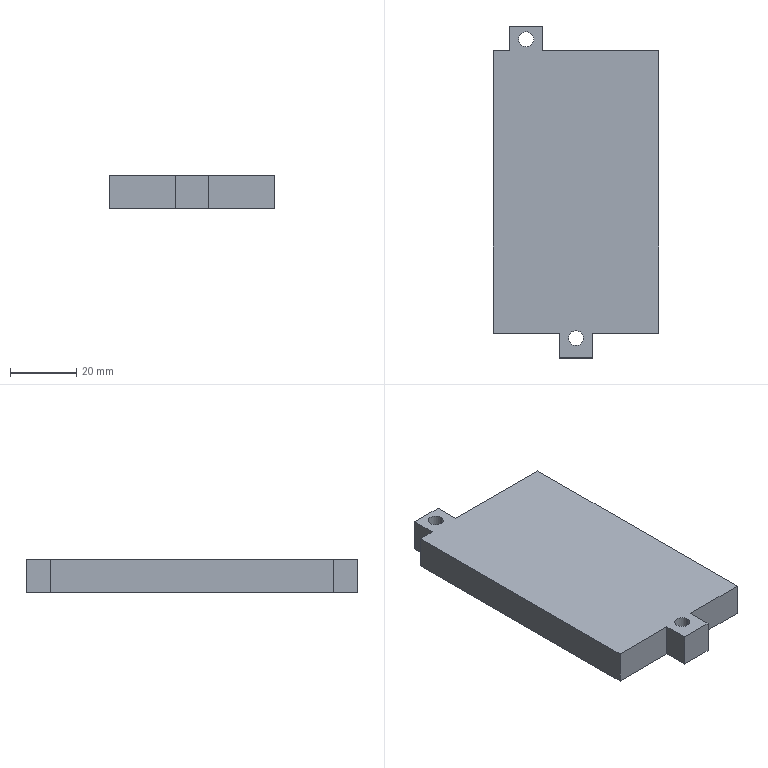Part | STEP file | Socket 1 | 1 solid | 18 faces | box 50 x 100 x 10 mm | volume 43682 mm3 | plane 14 | cylinder 4 | commonest cylinder face diameters 4.5 x4
STEP:
#1=CARTESIAN_POINT('',(0.,0.,0.));
#2=DIRECTION('',(0.,0.,1.));
#3=DIRECTION('',(1.,0.,0.));
#4=AXIS2_PLACEMENT_3D('',#1,#2,#3);
#5=CARTESIAN_POINT('',(-17.25,46.,10.));
#6=VERTEX_POINT('',#5);
#7=CARTESIAN_POINT('',(-17.25,46.,0.));
#8=VERTEX_POINT('',#7);
#9=CARTESIAN_POINT('',(-17.25,46.,10.));
#10=DIRECTION('',(0.,0.,-1.));
#11=VECTOR('',#10,1.);
#12=LINE('',#9,#11);
#13=CARTESIAN_POINT('',(-15.,46.,10.));
#14=DIRECTION('',(0.,0.,-1.));
#15=DIRECTION('',(-1.,0.,0.));
#16=AXIS2_PLACEMENT_3D('',#13,#14,#15);
#17=CYLINDRICAL_SURFACE('',#16,2.25);
#18=CARTESIAN_POINT('',(6.283,0.));
#19=DIRECTION('',(0.,1.));
#20=VECTOR('',#19,1.);
#21=LINE('',#18,#20);
#22=(GEOMETRIC_REPRESENTATION_CONTEXT(2)PARAMETRIC_REPRESENTATION_CONTEXT()REPRESENTATION_CONTEXT('',''));
#23=DEFINITIONAL_REPRESENTATION('',(#21),#22);
#24=PCURVE('',#17,#23);
#25=CARTESIAN_POINT('',(-15.,46.,10.));
#26=DIRECTION('',(0.,0.,-1.));
#27=DIRECTION('',(-1.,0.,0.));
#28=AXIS2_PLACEMENT_3D('',#25,#26,#27);
#29=CYLINDRICAL_SURFACE('',#28,2.25);
#30=CARTESIAN_POINT('',(0.,0.));
#31=DIRECTION('',(0.,1.));
#32=VECTOR('',#31,1.);
#33=LINE('',#30,#32);
#34=(GEOMETRIC_REPRESENTATION_CONTEXT(2)PARAMETRIC_REPRESENTATION_CONTEXT()REPRESENTATION_CONTEXT('',''));
#35=DEFINITIONAL_REPRESENTATION('',(#33),#34);
#36=PCURVE('',#29,#35);
#37=SURFACE_CURVE('',#12,(#24,#36),.PCURVE_S1.);
#38=EDGE_CURVE('',#6,#8,#37,.T.);
#39=ORIENTED_EDGE('',*,*,#38,.T.);
#40=CARTESIAN_POINT('',(-12.75,46.,0.));
#41=VERTEX_POINT('',#40);
#42=CARTESIAN_POINT('',(-15.,46.,0.));
#43=DIRECTION('',(0.,0.,1.));
#44=DIRECTION('',(-1.,0.,0.));
#45=AXIS2_PLACEMENT_3D('',#42,#43,#44);
#46=CIRCLE('',#45,2.25);
#47=CARTESIAN_POINT('',(6.283,10.));
#48=DIRECTION('',(-1.,0.));
#49=VECTOR('',#48,1.);
#50=LINE('',#47,#49);
#51=(GEOMETRIC_REPRESENTATION_CONTEXT(2)PARAMETRIC_REPRESENTATION_CONTEXT()REPRESENTATION_CONTEXT('',''));
#52=DEFINITIONAL_REPRESENTATION('',(#50),#51);
#53=PCURVE('',#17,#52);
#54=CARTESIAN_POINT('',(-1.349,-86.268,0.));
#55=DIRECTION('',(0.,0.,1.));
#56=DIRECTION('',(1.,0.,0.));
#57=AXIS2_PLACEMENT_3D('',#54,#55,#56);
#58=PLANE('',#57);
#59=CARTESIAN_POINT('',(-13.651,132.268));
#60=DIRECTION('',(-1.,0.));
#61=AXIS2_PLACEMENT_2D('',#59,#60);
#62=CIRCLE('',#61,2.25);
#63=(GEOMETRIC_REPRESENTATION_CONTEXT(2)PARAMETRIC_REPRESENTATION_CONTEXT()REPRESENTATION_CONTEXT('',''));
#64=DEFINITIONAL_REPRESENTATION('',(#62),#63);
#65=PCURVE('',#58,#64);
#66=SURFACE_CURVE('',#46,(#53,#65),.PCURVE_S1.);
#67=EDGE_CURVE('',#8,#41,#66,.T.);
#68=ORIENTED_EDGE('',*,*,#67,.T.);
#69=CARTESIAN_POINT('',(-12.75,46.,10.));
#70=VERTEX_POINT('',#69);
#71=CARTESIAN_POINT('',(-12.75,46.,10.));
#72=DIRECTION('',(0.,0.,-1.));
#73=VECTOR('',#72,1.);
#74=LINE('',#71,#73);
#75=CARTESIAN_POINT('',(3.142,0.));
#76=DIRECTION('',(0.,1.));
#77=VECTOR('',#76,1.);
#78=LINE('',#75,#77);
#79=(GEOMETRIC_REPRESENTATION_CONTEXT(2)PARAMETRIC_REPRESENTATION_CONTEXT()REPRESENTATION_CONTEXT('',''));
#80=DEFINITIONAL_REPRESENTATION('',(#78),#79);
#81=PCURVE('',#17,#80);
#82=CARTESIAN_POINT('',(3.142,0.));
#83=DIRECTION('',(0.,1.));
#84=VECTOR('',#83,1.);
#85=LINE('',#82,#84);
#86=(GEOMETRIC_REPRESENTATION_CONTEXT(2)PARAMETRIC_REPRESENTATION_CONTEXT()REPRESENTATION_CONTEXT('',''));
#87=DEFINITIONAL_REPRESENTATION('',(#85),#86);
#88=PCURVE('',#29,#87);
#89=SURFACE_CURVE('',#74,(#81,#88),.PCURVE_S1.);
#90=EDGE_CURVE('',#70,#41,#89,.T.);
#91=ORIENTED_EDGE('',*,*,#90,.F.);
#92=CARTESIAN_POINT('',(-15.,46.,10.));
#93=DIRECTION('',(0.,0.,-1.));
#94=DIRECTION('',(-1.,0.,0.));
#95=AXIS2_PLACEMENT_3D('',#92,#93,#94);
#96=CIRCLE('',#95,2.25);
#97=CARTESIAN_POINT('',(0.,0.));
#98=DIRECTION('',(1.,0.));
#99=VECTOR('',#98,1.);
#100=LINE('',#97,#99);
#101=(GEOMETRIC_REPRESENTATION_CONTEXT(2)PARAMETRIC_REPRESENTATION_CONTEXT()REPRESENTATION_CONTEXT('',''));
#102=DEFINITIONAL_REPRESENTATION('',(#100),#101);
#103=PCURVE('',#17,#102);
#104=CARTESIAN_POINT('',(-1.349,-86.268,10.));
#105=DIRECTION('',(0.,0.,1.));
#106=DIRECTION('',(1.,0.,0.));
#107=AXIS2_PLACEMENT_3D('',#104,#105,#106);
#108=PLANE('',#107);
#109=CARTESIAN_POINT('',(-15.901,132.268));
#110=CARTESIAN_POINT('',(-15.901,136.166));
#111=CARTESIAN_POINT('',(-12.526,134.217));
#112=CARTESIAN_POINT('',(-9.151,132.268));
#113=CARTESIAN_POINT('',(-12.526,130.32));
#114=CARTESIAN_POINT('',(-15.901,128.371));
#115=CARTESIAN_POINT('',(-15.901,132.268));
#116=(BOUNDED_CURVE()B_SPLINE_CURVE(2,(#109,#110,#111,#112,#113,#114,#115),.UNSPECIFIED.,.T.,.F.)B_SPLINE_CURVE_WITH_KNOTS((1,2,2,2,2,1),(-2.094,0.,2.094,4.189,6.283,8.378),.UNSPECIFIED.)CURVE()GEOMETRIC_REPRESENTATION_ITEM()RATIONAL_B_SPLINE_CURVE((1.,0.5,1.,0.5,1.,0.5,1.))REPRESENTATION_ITEM(''));
#117=(GEOMETRIC_REPRESENTATION_CONTEXT(2)PARAMETRIC_REPRESENTATION_CONTEXT()REPRESENTATION_CONTEXT('',''));
#118=DEFINITIONAL_REPRESENTATION('',(#116),#117);
#119=PCURVE('',#108,#118);
#120=SURFACE_CURVE('',#96,(#103,#119),.PCURVE_S1.);
#121=EDGE_CURVE('',#70,#6,#120,.T.);
#122=ORIENTED_EDGE('',*,*,#121,.T.);
#123=EDGE_LOOP('',(#39,#68,#91,#122));
#124=FACE_BOUND('',#123,.F.);
#125=ADVANCED_FACE('',(#124),#17,.F.);
#126=CARTESIAN_POINT('',(-2.25,-44.,10.));
#127=VERTEX_POINT('',#126);
#128=CARTESIAN_POINT('',(-2.25,-44.,0.));
#129=VERTEX_POINT('',#128);
#130=CARTESIAN_POINT('',(-2.25,-44.,10.));
#131=DIRECTION('',(0.,0.,-1.));
#132=VECTOR('',#131,1.);
#133=LINE('',#130,#132);
#134=CARTESIAN_POINT('',(0.,-44.,10.));
#135=DIRECTION('',(0.,0.,-1.));
#136=DIRECTION('',(-1.,0.,0.));
#137=AXIS2_PLACEMENT_3D('',#134,#135,#136);
#138=CYLINDRICAL_SURFACE('',#137,2.25);
#139=CARTESIAN_POINT('',(6.283,0.));
#140=DIRECTION('',(0.,1.));
#141=VECTOR('',#140,1.);
#142=LINE('',#139,#141);
#143=(GEOMETRIC_REPRESENTATION_CONTEXT(2)PARAMETRIC_REPRESENTATION_CONTEXT()REPRESENTATION_CONTEXT('',''));
#144=DEFINITIONAL_REPRESENTATION('',(#142),#143);
#145=PCURVE('',#138,#144);
#146=CARTESIAN_POINT('',(0.,-44.,10.));
#147=DIRECTION('',(0.,0.,-1.));
#148=DIRECTION('',(-1.,0.,0.));
#149=AXIS2_PLACEMENT_3D('',#146,#147,#148);
#150=CYLINDRICAL_SURFACE('',#149,2.25);
#151=CARTESIAN_POINT('',(0.,0.));
#152=DIRECTION('',(0.,1.));
#153=VECTOR('',#152,1.);
#154=LINE('',#151,#153);
#155=(GEOMETRIC_REPRESENTATION_CONTEXT(2)PARAMETRIC_REPRESENTATION_CONTEXT()REPRESENTATION_CONTEXT('',''));
#156=DEFINITIONAL_REPRESENTATION('',(#154),#155);
#157=PCURVE('',#150,#156);
#158=SURFACE_CURVE('',#133,(#145,#157),.PCURVE_S1.);
#159=EDGE_CURVE('',#127,#129,#158,.T.);
#160=ORIENTED_EDGE('',*,*,#159,.T.);
#161=CARTESIAN_POINT('',(2.25,-44.,0.));
#162=VERTEX_POINT('',#161);
#163=CARTESIAN_POINT('',(0.,-44.,0.));
#164=DIRECTION('',(0.,0.,1.));
#165=DIRECTION('',(-1.,0.,0.));
#166=AXIS2_PLACEMENT_3D('',#163,#164,#165);
#167=CIRCLE('',#166,2.25);
#168=CARTESIAN_POINT('',(6.283,10.));
#169=DIRECTION('',(-1.,0.));
#170=VECTOR('',#169,1.);
#171=LINE('',#168,#170);
#172=(GEOMETRIC_REPRESENTATION_CONTEXT(2)PARAMETRIC_REPRESENTATION_CONTEXT()REPRESENTATION_CONTEXT('',''));
#173=DEFINITIONAL_REPRESENTATION('',(#171),#172);
#174=PCURVE('',#138,#173);
#175=CARTESIAN_POINT('',(1.349,42.268));
#176=DIRECTION('',(-1.,0.));
#177=AXIS2_PLACEMENT_2D('',#175,#176);
#178=CIRCLE('',#177,2.25);
#179=(GEOMETRIC_REPRESENTATION_CONTEXT(2)PARAMETRIC_REPRESENTATION_CONTEXT()REPRESENTATION_CONTEXT('',''));
#180=DEFINITIONAL_REPRESENTATION('',(#178),#179);
#181=PCURVE('',#58,#180);
#182=SURFACE_CURVE('',#167,(#174,#181),.PCURVE_S1.);
#183=EDGE_CURVE('',#129,#162,#182,.T.);
#184=ORIENTED_EDGE('',*,*,#183,.T.);
#185=CARTESIAN_POINT('',(2.25,-44.,10.));
#186=VERTEX_POINT('',#185);
#187=CARTESIAN_POINT('',(2.25,-44.,10.));
#188=DIRECTION('',(0.,0.,-1.));
#189=VECTOR('',#188,1.);
#190=LINE('',#187,#189);
#191=CARTESIAN_POINT('',(3.142,0.));
#192=DIRECTION('',(0.,1.));
#193=VECTOR('',#192,1.);
#194=LINE('',#191,#193);
#195=(GEOMETRIC_REPRESENTATION_CONTEXT(2)PARAMETRIC_REPRESENTATION_CONTEXT()REPRESENTATION_CONTEXT('',''));
#196=DEFINITIONAL_REPRESENTATION('',(#194),#195);
#197=PCURVE('',#138,#196);
#198=CARTESIAN_POINT('',(3.142,0.));
#199=DIRECTION('',(0.,1.));
#200=VECTOR('',#199,1.);
#201=LINE('',#198,#200);
#202=(GEOMETRIC_REPRESENTATION_CONTEXT(2)PARAMETRIC_REPRESENTATION_CONTEXT()REPRESENTATION_CONTEXT('',''));
#203=DEFINITIONAL_REPRESENTATION('',(#201),#202);
#204=PCURVE('',#150,#203);
#205=SURFACE_CURVE('',#190,(#197,#204),.PCURVE_S1.);
#206=EDGE_CURVE('',#186,#162,#205,.T.);
#207=ORIENTED_EDGE('',*,*,#206,.F.);
#208=CARTESIAN_POINT('',(0.,-44.,10.));
#209=DIRECTION('',(0.,0.,-1.));
#210=DIRECTION('',(-1.,0.,0.));
#211=AXIS2_PLACEMENT_3D('',#208,#209,#210);
#212=CIRCLE('',#211,2.25);
#213=CARTESIAN_POINT('',(0.,0.));
#214=DIRECTION('',(1.,0.));
#215=VECTOR('',#214,1.);
#216=LINE('',#213,#215);
#217=(GEOMETRIC_REPRESENTATION_CONTEXT(2)PARAMETRIC_REPRESENTATION_CONTEXT()REPRESENTATION_CONTEXT('',''));
#218=DEFINITIONAL_REPRESENTATION('',(#216),#217);
#219=PCURVE('',#138,#218);
#220=CARTESIAN_POINT('',(-0.9015,42.268));
#221=CARTESIAN_POINT('',(-0.9015,46.166));
#222=CARTESIAN_POINT('',(2.474,44.217));
#223=CARTESIAN_POINT('',(5.849,42.268));
#224=CARTESIAN_POINT('',(2.474,40.32));
#225=CARTESIAN_POINT('',(-0.9015,38.371));
#226=CARTESIAN_POINT('',(-0.9015,42.268));
#227=(BOUNDED_CURVE()B_SPLINE_CURVE(2,(#220,#221,#222,#223,#224,#225,#226),.UNSPECIFIED.,.T.,.F.)B_SPLINE_CURVE_WITH_KNOTS((1,2,2,2,2,1),(-2.094,0.,2.094,4.189,6.283,8.378),.UNSPECIFIED.)CURVE()GEOMETRIC_REPRESENTATION_ITEM()RATIONAL_B_SPLINE_CURVE((1.,0.5,1.,0.5,1.,0.5,1.))REPRESENTATION_ITEM(''));
#228=(GEOMETRIC_REPRESENTATION_CONTEXT(2)PARAMETRIC_REPRESENTATION_CONTEXT()REPRESENTATION_CONTEXT('',''));
#229=DEFINITIONAL_REPRESENTATION('',(#227),#228);
#230=PCURVE('',#108,#229);
#231=SURFACE_CURVE('',#212,(#219,#230),.PCURVE_S1.);
#232=EDGE_CURVE('',#186,#127,#231,.T.);
#233=ORIENTED_EDGE('',*,*,#232,.T.);
#234=EDGE_LOOP('',(#160,#184,#207,#233));
#235=FACE_BOUND('',#234,.F.);
#236=ADVANCED_FACE('',(#235),#138,.F.);
#237=CARTESIAN_POINT('',(-15.,46.,10.));
#238=DIRECTION('',(0.,0.,-1.));
#239=DIRECTION('',(-1.,0.,0.));
#240=AXIS2_PLACEMENT_3D('',#237,#238,#239);
#241=CIRCLE('',#240,2.25);
#242=CARTESIAN_POINT('',(-15.901,132.268));
#243=CARTESIAN_POINT('',(-15.901,136.166));
#244=CARTESIAN_POINT('',(-12.526,134.217));
#245=CARTESIAN_POINT('',(-9.151,132.268));
#246=CARTESIAN_POINT('',(-12.526,130.32));
#247=CARTESIAN_POINT('',(-15.901,128.371));
#248=CARTESIAN_POINT('',(-15.901,132.268));
#249=(BOUNDED_CURVE()B_SPLINE_CURVE(2,(#242,#243,#244,#245,#246,#247,#248),.UNSPECIFIED.,.T.,.F.)B_SPLINE_CURVE_WITH_KNOTS((1,2,2,2,2,1),(-2.094,0.,2.094,4.189,6.283,8.378),.UNSPECIFIED.)CURVE()GEOMETRIC_REPRESENTATION_ITEM()RATIONAL_B_SPLINE_CURVE((1.,0.5,1.,0.5,1.,0.5,1.))REPRESENTATION_ITEM(''));
#250=(GEOMETRIC_REPRESENTATION_CONTEXT(2)PARAMETRIC_REPRESENTATION_CONTEXT()REPRESENTATION_CONTEXT('',''));
#251=DEFINITIONAL_REPRESENTATION('',(#249),#250);
#252=PCURVE('',#108,#251);
#253=CARTESIAN_POINT('',(0.,0.));
#254=DIRECTION('',(1.,0.));
#255=VECTOR('',#254,1.);
#256=LINE('',#253,#255);
#257=(GEOMETRIC_REPRESENTATION_CONTEXT(2)PARAMETRIC_REPRESENTATION_CONTEXT()REPRESENTATION_CONTEXT('',''));
#258=DEFINITIONAL_REPRESENTATION('',(#256),#257);
#259=PCURVE('',#29,#258);
#260=SURFACE_CURVE('',#241,(#252,#259),.PCURVE_S1.);
#261=EDGE_CURVE('',#6,#70,#260,.T.);
#262=ORIENTED_EDGE('',*,*,#261,.T.);
#263=ORIENTED_EDGE('',*,*,#121,.T.);
#264=EDGE_LOOP('',(#262,#263));
#265=FACE_BOUND('',#264,.T.);
#266=CARTESIAN_POINT('',(0.,-44.,10.));
#267=DIRECTION('',(0.,0.,-1.));
#268=DIRECTION('',(-1.,0.,0.));
#269=AXIS2_PLACEMENT_3D('',#266,#267,#268);
#270=CIRCLE('',#269,2.25);
#271=CARTESIAN_POINT('',(-0.9015,42.268));
#272=CARTESIAN_POINT('',(-0.9015,46.166));
#273=CARTESIAN_POINT('',(2.474,44.217));
#274=CARTESIAN_POINT('',(5.849,42.268));
#275=CARTESIAN_POINT('',(2.474,40.32));
#276=CARTESIAN_POINT('',(-0.9015,38.371));
#277=CARTESIAN_POINT('',(-0.9015,42.268));
#278=(BOUNDED_CURVE()B_SPLINE_CURVE(2,(#271,#272,#273,#274,#275,#276,#277),.UNSPECIFIED.,.T.,.F.)B_SPLINE_CURVE_WITH_KNOTS((1,2,2,2,2,1),(-2.094,0.,2.094,4.189,6.283,8.378),.UNSPECIFIED.)CURVE()GEOMETRIC_REPRESENTATION_ITEM()RATIONAL_B_SPLINE_CURVE((1.,0.5,1.,0.5,1.,0.5,1.))REPRESENTATION_ITEM(''));
#279=(GEOMETRIC_REPRESENTATION_CONTEXT(2)PARAMETRIC_REPRESENTATION_CONTEXT()REPRESENTATION_CONTEXT('',''));
#280=DEFINITIONAL_REPRESENTATION('',(#278),#279);
#281=PCURVE('',#108,#280);
#282=CARTESIAN_POINT('',(0.,0.));
#283=DIRECTION('',(1.,0.));
#284=VECTOR('',#283,1.);
#285=LINE('',#282,#284);
#286=(GEOMETRIC_REPRESENTATION_CONTEXT(2)PARAMETRIC_REPRESENTATION_CONTEXT()REPRESENTATION_CONTEXT('',''));
#287=DEFINITIONAL_REPRESENTATION('',(#285),#286);
#288=PCURVE('',#150,#287);
#289=SURFACE_CURVE('',#270,(#281,#288),.PCURVE_S1.);
#290=EDGE_CURVE('',#127,#186,#289,.T.);
#291=ORIENTED_EDGE('',*,*,#290,.T.);
#292=ORIENTED_EDGE('',*,*,#232,.T.);
#293=EDGE_LOOP('',(#291,#292));
#294=FACE_BOUND('',#293,.T.);
#295=CARTESIAN_POINT('',(-5.,-42.5,10.));
#296=VERTEX_POINT('',#295);
#297=CARTESIAN_POINT('',(-5.,-50.,10.));
#298=VERTEX_POINT('',#297);
#299=CARTESIAN_POINT('',(-5.,-86.268,10.));
#300=DIRECTION('',(0.,-1.,0.));
#301=VECTOR('',#300,1.);
#302=LINE('',#299,#301);
#303=CARTESIAN_POINT('',(-3.651,0.));
#304=DIRECTION('',(0.,-1.));
#305=VECTOR('',#304,1.);
#306=LINE('',#303,#305);
#307=(GEOMETRIC_REPRESENTATION_CONTEXT(2)PARAMETRIC_REPRESENTATION_CONTEXT()REPRESENTATION_CONTEXT('',''));
#308=DEFINITIONAL_REPRESENTATION('',(#306),#307);
#309=PCURVE('',#108,#308);
#310=CARTESIAN_POINT('',(-5.,-86.268,10.));
#311=DIRECTION('',(1.,0.,0.));
#312=DIRECTION('',(0.,1.,0.));
#313=AXIS2_PLACEMENT_3D('',#310,#311,#312);
#314=PLANE('',#313);
#315=CARTESIAN_POINT('',(0.,0.));
#316=DIRECTION('',(-1.,0.));
#317=VECTOR('',#316,1.);
#318=LINE('',#315,#317);
#319=(GEOMETRIC_REPRESENTATION_CONTEXT(2)PARAMETRIC_REPRESENTATION_CONTEXT()REPRESENTATION_CONTEXT('',''));
#320=DEFINITIONAL_REPRESENTATION('',(#318),#319);
#321=PCURVE('',#314,#320);
#322=SURFACE_CURVE('',#302,(#309,#321),.PCURVE_S1.);
#323=EDGE_CURVE('',#296,#298,#322,.T.);
#324=ORIENTED_EDGE('',*,*,#323,.T.);
#325=CARTESIAN_POINT('',(5.,-50.,10.));
#326=VERTEX_POINT('',#325);
#327=CARTESIAN_POINT('',(-1.349,-50.,10.));
#328=DIRECTION('',(1.,0.,0.));
#329=VECTOR('',#328,1.);
#330=LINE('',#327,#329);
#331=CARTESIAN_POINT('',(0.,36.268));
#332=DIRECTION('',(1.,0.));
#333=VECTOR('',#332,1.);
#334=LINE('',#331,#333);
#335=(GEOMETRIC_REPRESENTATION_CONTEXT(2)PARAMETRIC_REPRESENTATION_CONTEXT()REPRESENTATION_CONTEXT('',''));
#336=DEFINITIONAL_REPRESENTATION('',(#334),#335);
#337=PCURVE('',#108,#336);
#338=CARTESIAN_POINT('',(-1.349,-50.,10.));
#339=DIRECTION('',(0.,1.,0.));
#340=DIRECTION('',(0.,0.,1.));
#341=AXIS2_PLACEMENT_3D('',#338,#339,#340);
#342=PLANE('',#341);
#343=CARTESIAN_POINT('',(0.,0.));
#344=DIRECTION('',(0.,1.));
#345=VECTOR('',#344,1.);
#346=LINE('',#343,#345);
#347=(GEOMETRIC_REPRESENTATION_CONTEXT(2)PARAMETRIC_REPRESENTATION_CONTEXT()REPRESENTATION_CONTEXT('',''));
#348=DEFINITIONAL_REPRESENTATION('',(#346),#347);
#349=PCURVE('',#342,#348);
#350=SURFACE_CURVE('',#330,(#337,#349),.PCURVE_S1.);
#351=EDGE_CURVE('',#298,#326,#350,.T.);
#352=ORIENTED_EDGE('',*,*,#351,.T.);
#353=CARTESIAN_POINT('',(5.,-42.5,10.));
#354=VERTEX_POINT('',#353);
#355=CARTESIAN_POINT('',(5.,-86.268,10.));
#356=DIRECTION('',(0.,1.,0.));
#357=VECTOR('',#356,1.);
#358=LINE('',#355,#357);
#359=CARTESIAN_POINT('',(6.349,0.));
#360=DIRECTION('',(0.,1.));
#361=VECTOR('',#360,1.);
#362=LINE('',#359,#361);
#363=(GEOMETRIC_REPRESENTATION_CONTEXT(2)PARAMETRIC_REPRESENTATION_CONTEXT()REPRESENTATION_CONTEXT('',''));
#364=DEFINITIONAL_REPRESENTATION('',(#362),#363);
#365=PCURVE('',#108,#364);
#366=CARTESIAN_POINT('',(5.,-86.268,10.));
#367=DIRECTION('',(1.,0.,0.));
#368=DIRECTION('',(0.,1.,0.));
#369=AXIS2_PLACEMENT_3D('',#366,#367,#368);
#370=PLANE('',#369);
#371=CARTESIAN_POINT('',(0.,0.));
#372=DIRECTION('',(1.,0.));
#373=VECTOR('',#372,1.);
#374=LINE('',#371,#373);
#375=(GEOMETRIC_REPRESENTATION_CONTEXT(2)PARAMETRIC_REPRESENTATION_CONTEXT()REPRESENTATION_CONTEXT('',''));
#376=DEFINITIONAL_REPRESENTATION('',(#374),#375);
#377=PCURVE('',#370,#376);
#378=SURFACE_CURVE('',#358,(#365,#377),.PCURVE_S1.);
#379=EDGE_CURVE('',#326,#354,#378,.T.);
#380=ORIENTED_EDGE('',*,*,#379,.T.);
#381=CARTESIAN_POINT('',(25.,-42.5,10.));
#382=VERTEX_POINT('',#381);
#383=CARTESIAN_POINT('',(-1.349,-42.5,10.));
#384=DIRECTION('',(1.,0.,0.));
#385=VECTOR('',#384,1.);
#386=LINE('',#383,#385);
#387=CARTESIAN_POINT('',(0.,43.768));
#388=DIRECTION('',(1.,0.));
#389=VECTOR('',#388,1.);
#390=LINE('',#387,#389);
#391=(GEOMETRIC_REPRESENTATION_CONTEXT(2)PARAMETRIC_REPRESENTATION_CONTEXT()REPRESENTATION_CONTEXT('',''));
#392=DEFINITIONAL_REPRESENTATION('',(#390),#391);
#393=PCURVE('',#108,#392);
#394=CARTESIAN_POINT('',(-1.349,-42.5,10.));
#395=DIRECTION('',(0.,1.,0.));
#396=DIRECTION('',(0.,0.,1.));
#397=AXIS2_PLACEMENT_3D('',#394,#395,#396);
#398=PLANE('',#397);
#399=CARTESIAN_POINT('',(0.,0.));
#400=DIRECTION('',(0.,1.));
#401=VECTOR('',#400,1.);
#402=LINE('',#399,#401);
#403=(GEOMETRIC_REPRESENTATION_CONTEXT(2)PARAMETRIC_REPRESENTATION_CONTEXT()REPRESENTATION_CONTEXT('',''));
#404=DEFINITIONAL_REPRESENTATION('',(#402),#403);
#405=PCURVE('',#398,#404);
#406=SURFACE_CURVE('',#386,(#393,#405),.PCURVE_S1.);
#407=EDGE_CURVE('',#354,#382,#406,.T.);
#408=ORIENTED_EDGE('',*,*,#407,.T.);
#409=CARTESIAN_POINT('',(25.,42.5,10.));
#410=VERTEX_POINT('',#409);
#411=CARTESIAN_POINT('',(25.,-86.268,10.));
#412=DIRECTION('',(0.,1.,0.));
#413=VECTOR('',#412,1.);
#414=LINE('',#411,#413);
#415=CARTESIAN_POINT('',(26.349,0.));
#416=DIRECTION('',(0.,1.));
#417=VECTOR('',#416,1.);
#418=LINE('',#415,#417);
#419=(GEOMETRIC_REPRESENTATION_CONTEXT(2)PARAMETRIC_REPRESENTATION_CONTEXT()REPRESENTATION_CONTEXT('',''));
#420=DEFINITIONAL_REPRESENTATION('',(#418),#419);
#421=PCURVE('',#108,#420);
#422=CARTESIAN_POINT('',(25.,-86.268,10.));
#423=DIRECTION('',(1.,0.,0.));
#424=DIRECTION('',(0.,1.,0.));
#425=AXIS2_PLACEMENT_3D('',#422,#423,#424);
#426=PLANE('',#425);
#427=CARTESIAN_POINT('',(0.,0.));
#428=DIRECTION('',(1.,0.));
#429=VECTOR('',#428,1.);
#430=LINE('',#427,#429);
#431=(GEOMETRIC_REPRESENTATION_CONTEXT(2)PARAMETRIC_REPRESENTATION_CONTEXT()REPRESENTATION_CONTEXT('',''));
#432=DEFINITIONAL_REPRESENTATION('',(#430),#431);
#433=PCURVE('',#426,#432);
#434=SURFACE_CURVE('',#414,(#421,#433),.PCURVE_S1.);
#435=EDGE_CURVE('',#382,#410,#434,.T.);
#436=ORIENTED_EDGE('',*,*,#435,.T.);
#437=CARTESIAN_POINT('',(-10.,42.5,10.));
#438=VERTEX_POINT('',#437);
#439=CARTESIAN_POINT('',(-1.349,42.5,10.));
#440=DIRECTION('',(-1.,0.,0.));
#441=VECTOR('',#440,1.);
#442=LINE('',#439,#441);
#443=CARTESIAN_POINT('',(0.,128.768));
#444=DIRECTION('',(-1.,0.));
#445=VECTOR('',#444,1.);
#446=LINE('',#443,#445);
#447=(GEOMETRIC_REPRESENTATION_CONTEXT(2)PARAMETRIC_REPRESENTATION_CONTEXT()REPRESENTATION_CONTEXT('',''));
#448=DEFINITIONAL_REPRESENTATION('',(#446),#447);
#449=PCURVE('',#108,#448);
#450=CARTESIAN_POINT('',(-1.349,42.5,10.));
#451=DIRECTION('',(0.,1.,0.));
#452=DIRECTION('',(0.,0.,1.));
#453=AXIS2_PLACEMENT_3D('',#450,#451,#452);
#454=PLANE('',#453);
#455=CARTESIAN_POINT('',(0.,0.));
#456=DIRECTION('',(0.,-1.));
#457=VECTOR('',#456,1.);
#458=LINE('',#455,#457);
#459=(GEOMETRIC_REPRESENTATION_CONTEXT(2)PARAMETRIC_REPRESENTATION_CONTEXT()REPRESENTATION_CONTEXT('',''));
#460=DEFINITIONAL_REPRESENTATION('',(#458),#459);
#461=PCURVE('',#454,#460);
#462=SURFACE_CURVE('',#442,(#449,#461),.PCURVE_S1.);
#463=EDGE_CURVE('',#410,#438,#462,.T.);
#464=ORIENTED_EDGE('',*,*,#463,.T.);
#465=CARTESIAN_POINT('',(-10.,50.,10.));
#466=VERTEX_POINT('',#465);
#467=CARTESIAN_POINT('',(-10.,-86.268,10.));
#468=DIRECTION('',(0.,1.,0.));
#469=VECTOR('',#468,1.);
#470=LINE('',#467,#469);
#471=CARTESIAN_POINT('',(-8.651,0.));
#472=DIRECTION('',(0.,1.));
#473=VECTOR('',#472,1.);
#474=LINE('',#471,#473);
#475=(GEOMETRIC_REPRESENTATION_CONTEXT(2)PARAMETRIC_REPRESENTATION_CONTEXT()REPRESENTATION_CONTEXT('',''));
#476=DEFINITIONAL_REPRESENTATION('',(#474),#475);
#477=PCURVE('',#108,#476);
#478=CARTESIAN_POINT('',(-10.,-86.268,10.));
#479=DIRECTION('',(-1.,0.,0.));
#480=DIRECTION('',(0.,-1.,0.));
#481=AXIS2_PLACEMENT_3D('',#478,#479,#480);
#482=PLANE('',#481);
#483=CARTESIAN_POINT('',(0.,0.));
#484=DIRECTION('',(-1.,0.));
#485=VECTOR('',#484,1.);
#486=LINE('',#483,#485);
#487=(GEOMETRIC_REPRESENTATION_CONTEXT(2)PARAMETRIC_REPRESENTATION_CONTEXT()REPRESENTATION_CONTEXT('',''));
#488=DEFINITIONAL_REPRESENTATION('',(#486),#487);
#489=PCURVE('',#482,#488);
#490=SURFACE_CURVE('',#470,(#477,#489),.PCURVE_S1.);
#491=EDGE_CURVE('',#438,#466,#490,.T.);
#492=ORIENTED_EDGE('',*,*,#491,.T.);
#493=CARTESIAN_POINT('',(-20.,50.,10.));
#494=VERTEX_POINT('',#493);
#495=CARTESIAN_POINT('',(-1.349,50.,10.));
#496=DIRECTION('',(-1.,0.,0.));
#497=VECTOR('',#496,1.);
#498=LINE('',#495,#497);
#499=CARTESIAN_POINT('',(0.,136.268));
#500=DIRECTION('',(-1.,0.));
#501=VECTOR('',#500,1.);
#502=LINE('',#499,#501);
#503=(GEOMETRIC_REPRESENTATION_CONTEXT(2)PARAMETRIC_REPRESENTATION_CONTEXT()REPRESENTATION_CONTEXT('',''));
#504=DEFINITIONAL_REPRESENTATION('',(#502),#503);
#505=PCURVE('',#108,#504);
#506=CARTESIAN_POINT('',(-1.349,50.,10.));
#507=DIRECTION('',(0.,1.,0.));
#508=DIRECTION('',(0.,0.,1.));
#509=AXIS2_PLACEMENT_3D('',#506,#507,#508);
#510=PLANE('',#509);
#511=CARTESIAN_POINT('',(0.,0.));
#512=DIRECTION('',(0.,-1.));
#513=VECTOR('',#512,1.);
#514=LINE('',#511,#513);
#515=(GEOMETRIC_REPRESENTATION_CONTEXT(2)PARAMETRIC_REPRESENTATION_CONTEXT()REPRESENTATION_CONTEXT('',''));
#516=DEFINITIONAL_REPRESENTATION('',(#514),#515);
#517=PCURVE('',#510,#516);
#518=SURFACE_CURVE('',#498,(#505,#517),.PCURVE_S1.);
#519=EDGE_CURVE('',#466,#494,#518,.T.);
#520=ORIENTED_EDGE('',*,*,#519,.T.);
#521=CARTESIAN_POINT('',(-20.,42.5,10.));
#522=VERTEX_POINT('',#521);
#523=CARTESIAN_POINT('',(-20.,-86.268,10.));
#524=DIRECTION('',(0.,-1.,0.));
#525=VECTOR('',#524,1.);
#526=LINE('',#523,#525);
#527=CARTESIAN_POINT('',(-18.651,0.));
#528=DIRECTION('',(0.,-1.));
#529=VECTOR('',#528,1.);
#530=LINE('',#527,#529);
#531=(GEOMETRIC_REPRESENTATION_CONTEXT(2)PARAMETRIC_REPRESENTATION_CONTEXT()REPRESENTATION_CONTEXT('',''));
#532=DEFINITIONAL_REPRESENTATION('',(#530),#531);
#533=PCURVE('',#108,#532);
#534=CARTESIAN_POINT('',(-20.,-86.268,10.));
#535=DIRECTION('',(-1.,0.,0.));
#536=DIRECTION('',(0.,0.,1.));
#537=AXIS2_PLACEMENT_3D('',#534,#535,#536);
#538=PLANE('',#537);
#539=CARTESIAN_POINT('',(0.,0.));
#540=DIRECTION('',(0.,-1.));
#541=VECTOR('',#540,1.);
#542=LINE('',#539,#541);
#543=(GEOMETRIC_REPRESENTATION_CONTEXT(2)PARAMETRIC_REPRESENTATION_CONTEXT()REPRESENTATION_CONTEXT('',''));
#544=DEFINITIONAL_REPRESENTATION('',(#542),#543);
#545=PCURVE('',#538,#544);
#546=SURFACE_CURVE('',#526,(#533,#545),.PCURVE_S1.);
#547=EDGE_CURVE('',#494,#522,#546,.T.);
#548=ORIENTED_EDGE('',*,*,#547,.T.);
#549=CARTESIAN_POINT('',(-25.,42.5,10.));
#550=VERTEX_POINT('',#549);
#551=CARTESIAN_POINT('',(-1.349,42.5,10.));
#552=DIRECTION('',(-1.,0.,0.));
#553=VECTOR('',#552,1.);
#554=LINE('',#551,#553);
#555=CARTESIAN_POINT('',(0.,128.768));
#556=DIRECTION('',(-1.,0.));
#557=VECTOR('',#556,1.);
#558=LINE('',#555,#557);
#559=(GEOMETRIC_REPRESENTATION_CONTEXT(2)PARAMETRIC_REPRESENTATION_CONTEXT()REPRESENTATION_CONTEXT('',''));
#560=DEFINITIONAL_REPRESENTATION('',(#558),#559);
#561=PCURVE('',#108,#560);
#562=CARTESIAN_POINT('',(-1.349,42.5,10.));
#563=DIRECTION('',(0.,1.,0.));
#564=DIRECTION('',(0.,0.,1.));
#565=AXIS2_PLACEMENT_3D('',#562,#563,#564);
#566=PLANE('',#565);
#567=CARTESIAN_POINT('',(0.,0.));
#568=DIRECTION('',(0.,-1.));
#569=VECTOR('',#568,1.);
#570=LINE('',#567,#569);
#571=(GEOMETRIC_REPRESENTATION_CONTEXT(2)PARAMETRIC_REPRESENTATION_CONTEXT()REPRESENTATION_CONTEXT('',''));
#572=DEFINITIONAL_REPRESENTATION('',(#570),#571);
#573=PCURVE('',#566,#572);
#574=SURFACE_CURVE('',#554,(#561,#573),.PCURVE_S1.);
#575=EDGE_CURVE('',#522,#550,#574,.T.);
#576=ORIENTED_EDGE('',*,*,#575,.T.);
#577=CARTESIAN_POINT('',(-25.,-42.5,10.));
#578=VERTEX_POINT('',#577);
#579=CARTESIAN_POINT('',(-25.,-86.268,10.));
#580=DIRECTION('',(0.,-1.,0.));
#581=VECTOR('',#580,1.);
#582=LINE('',#579,#581);
#583=CARTESIAN_POINT('',(-23.651,0.));
#584=DIRECTION('',(0.,-1.));
#585=VECTOR('',#584,1.);
#586=LINE('',#583,#585);
#587=(GEOMETRIC_REPRESENTATION_CONTEXT(2)PARAMETRIC_REPRESENTATION_CONTEXT()REPRESENTATION_CONTEXT('',''));
#588=DEFINITIONAL_REPRESENTATION('',(#586),#587);
#589=PCURVE('',#108,#588);
#590=CARTESIAN_POINT('',(-25.,-86.268,10.));
#591=DIRECTION('',(1.,0.,0.));
#592=DIRECTION('',(0.,0.,-1.));
#593=AXIS2_PLACEMENT_3D('',#590,#591,#592);
#594=PLANE('',#593);
#595=CARTESIAN_POINT('',(0.,0.));
#596=DIRECTION('',(0.,-1.));
#597=VECTOR('',#596,1.);
#598=LINE('',#595,#597);
#599=(GEOMETRIC_REPRESENTATION_CONTEXT(2)PARAMETRIC_REPRESENTATION_CONTEXT()REPRESENTATION_CONTEXT('',''));
#600=DEFINITIONAL_REPRESENTATION('',(#598),#599);
#601=PCURVE('',#594,#600);
#602=SURFACE_CURVE('',#582,(#589,#601),.PCURVE_S1.);
#603=EDGE_CURVE('',#550,#578,#602,.T.);
#604=ORIENTED_EDGE('',*,*,#603,.T.);
#605=CARTESIAN_POINT('',(-1.349,-42.5,10.));
#606=DIRECTION('',(1.,0.,0.));
#607=VECTOR('',#606,1.);
#608=LINE('',#605,#607);
#609=CARTESIAN_POINT('',(0.,43.768));
#610=DIRECTION('',(1.,0.));
#611=VECTOR('',#610,1.);
#612=LINE('',#609,#611);
#613=(GEOMETRIC_REPRESENTATION_CONTEXT(2)PARAMETRIC_REPRESENTATION_CONTEXT()REPRESENTATION_CONTEXT('',''));
#614=DEFINITIONAL_REPRESENTATION('',(#612),#613);
#615=PCURVE('',#108,#614);
#616=CARTESIAN_POINT('',(-1.349,-42.5,10.));
#617=DIRECTION('',(0.,1.,0.));
#618=DIRECTION('',(0.,0.,1.));
#619=AXIS2_PLACEMENT_3D('',#616,#617,#618);
#620=PLANE('',#619);
#621=CARTESIAN_POINT('',(0.,0.));
#622=DIRECTION('',(0.,1.));
#623=VECTOR('',#622,1.);
#624=LINE('',#621,#623);
#625=(GEOMETRIC_REPRESENTATION_CONTEXT(2)PARAMETRIC_REPRESENTATION_CONTEXT()REPRESENTATION_CONTEXT('',''));
#626=DEFINITIONAL_REPRESENTATION('',(#624),#625);
#627=PCURVE('',#620,#626);
#628=SURFACE_CURVE('',#608,(#615,#627),.PCURVE_S1.);
#629=EDGE_CURVE('',#578,#296,#628,.T.);
#630=ORIENTED_EDGE('',*,*,#629,.T.);
#631=EDGE_LOOP('',(#324,#352,#380,#408,#436,#464,#492,#520,#548,#576,#604,#630));
#632=FACE_BOUND('',#631,.T.);
#633=ADVANCED_FACE('',(#265,#294,#632),#108,.T.);
#634=CARTESIAN_POINT('',(-15.,46.,0.));
#635=DIRECTION('',(0.,0.,1.));
#636=DIRECTION('',(-1.,0.,0.));
#637=AXIS2_PLACEMENT_3D('',#634,#635,#636);
#638=CIRCLE('',#637,2.25);
#639=CARTESIAN_POINT('',(6.283,10.));
#640=DIRECTION('',(-1.,0.));
#641=VECTOR('',#640,1.);
#642=LINE('',#639,#641);
#643=(GEOMETRIC_REPRESENTATION_CONTEXT(2)PARAMETRIC_REPRESENTATION_CONTEXT()REPRESENTATION_CONTEXT('',''));
#644=DEFINITIONAL_REPRESENTATION('',(#642),#643);
#645=PCURVE('',#29,#644);
#646=CARTESIAN_POINT('',(-13.651,132.268));
#647=DIRECTION('',(-1.,0.));
#648=AXIS2_PLACEMENT_2D('',#646,#647);
#649=CIRCLE('',#648,2.25);
#650=(GEOMETRIC_REPRESENTATION_CONTEXT(2)PARAMETRIC_REPRESENTATION_CONTEXT()REPRESENTATION_CONTEXT('',''));
#651=DEFINITIONAL_REPRESENTATION('',(#649),#650);
#652=PCURVE('',#58,#651);
#653=SURFACE_CURVE('',#638,(#645,#652),.PCURVE_S1.);
#654=EDGE_CURVE('',#41,#8,#653,.T.);
#655=ORIENTED_EDGE('',*,*,#654,.T.);
#656=ORIENTED_EDGE('',*,*,#38,.F.);
#657=ORIENTED_EDGE('',*,*,#261,.T.);
#658=ORIENTED_EDGE('',*,*,#90,.T.);
#659=EDGE_LOOP('',(#655,#656,#657,#658));
#660=FACE_BOUND('',#659,.F.);
#661=ADVANCED_FACE('',(#660),#29,.F.);
#662=CARTESIAN_POINT('',(0.,-44.,0.));
#663=DIRECTION('',(0.,0.,1.));
#664=DIRECTION('',(-1.,0.,0.));
#665=AXIS2_PLACEMENT_3D('',#662,#663,#664);
#666=CIRCLE('',#665,2.25);
#667=CARTESIAN_POINT('',(6.283,10.));
#668=DIRECTION('',(-1.,0.));
#669=VECTOR('',#668,1.);
#670=LINE('',#667,#669);
#671=(GEOMETRIC_REPRESENTATION_CONTEXT(2)PARAMETRIC_REPRESENTATION_CONTEXT()REPRESENTATION_CONTEXT('',''));
#672=DEFINITIONAL_REPRESENTATION('',(#670),#671);
#673=PCURVE('',#150,#672);
#674=CARTESIAN_POINT('',(1.349,42.268));
#675=DIRECTION('',(-1.,0.));
#676=AXIS2_PLACEMENT_2D('',#674,#675);
#677=CIRCLE('',#676,2.25);
#678=(GEOMETRIC_REPRESENTATION_CONTEXT(2)PARAMETRIC_REPRESENTATION_CONTEXT()REPRESENTATION_CONTEXT('',''));
#679=DEFINITIONAL_REPRESENTATION('',(#677),#678);
#680=PCURVE('',#58,#679);
#681=SURFACE_CURVE('',#666,(#673,#680),.PCURVE_S1.);
#682=EDGE_CURVE('',#162,#129,#681,.T.);
#683=ORIENTED_EDGE('',*,*,#682,.T.);
#684=ORIENTED_EDGE('',*,*,#159,.F.);
#685=ORIENTED_EDGE('',*,*,#290,.T.);
#686=ORIENTED_EDGE('',*,*,#206,.T.);
#687=EDGE_LOOP('',(#683,#684,#685,#686));
#688=FACE_BOUND('',#687,.F.);
#689=ADVANCED_FACE('',(#688),#150,.F.);
#690=CARTESIAN_POINT('',(5.,-50.,0.));
#691=VERTEX_POINT('',#690);
#692=CARTESIAN_POINT('',(5.,-50.,10.));
#693=DIRECTION('',(0.,0.,-1.));
#694=VECTOR('',#693,1.);
#695=LINE('',#692,#694);
#696=CARTESIAN_POINT('',(0.,6.349));
#697=DIRECTION('',(-1.,0.));
#698=VECTOR('',#697,1.);
#699=LINE('',#696,#698);
#700=(GEOMETRIC_REPRESENTATION_CONTEXT(2)PARAMETRIC_REPRESENTATION_CONTEXT()REPRESENTATION_CONTEXT('',''));
#701=DEFINITIONAL_REPRESENTATION('',(#699),#700);
#702=PCURVE('',#342,#701);
#703=CARTESIAN_POINT('',(36.268,0.));
#704=DIRECTION('',(0.,-1.));
#705=VECTOR('',#704,1.);
#706=LINE('',#703,#705);
#707=(GEOMETRIC_REPRESENTATION_CONTEXT(2)PARAMETRIC_REPRESENTATION_CONTEXT()REPRESENTATION_CONTEXT('',''));
#708=DEFINITIONAL_REPRESENTATION('',(#706),#707);
#709=PCURVE('',#370,#708);
#710=SURFACE_CURVE('',#695,(#702,#709),.PCURVE_S1.);
#711=EDGE_CURVE('',#326,#691,#710,.T.);
#712=ORIENTED_EDGE('',*,*,#711,.F.);
#713=ORIENTED_EDGE('',*,*,#351,.F.);
#714=CARTESIAN_POINT('',(-5.,-50.,0.));
#715=VERTEX_POINT('',#714);
#716=CARTESIAN_POINT('',(-5.,-50.,10.));
#717=DIRECTION('',(0.,0.,1.));
#718=VECTOR('',#717,1.);
#719=LINE('',#716,#718);
#720=CARTESIAN_POINT('',(0.,-3.651));
#721=DIRECTION('',(1.,0.));
#722=VECTOR('',#721,1.);
#723=LINE('',#720,#722);
#724=(GEOMETRIC_REPRESENTATION_CONTEXT(2)PARAMETRIC_REPRESENTATION_CONTEXT()REPRESENTATION_CONTEXT('',''));
#725=DEFINITIONAL_REPRESENTATION('',(#723),#724);
#726=PCURVE('',#342,#725);
#727=CARTESIAN_POINT('',(36.268,0.));
#728=DIRECTION('',(0.,1.));
#729=VECTOR('',#728,1.);
#730=LINE('',#727,#729);
#731=(GEOMETRIC_REPRESENTATION_CONTEXT(2)PARAMETRIC_REPRESENTATION_CONTEXT()REPRESENTATION_CONTEXT('',''));
#732=DEFINITIONAL_REPRESENTATION('',(#730),#731);
#733=PCURVE('',#314,#732);
#734=SURFACE_CURVE('',#719,(#726,#733),.PCURVE_S1.);
#735=EDGE_CURVE('',#715,#298,#734,.T.);
#736=ORIENTED_EDGE('',*,*,#735,.F.);
#737=CARTESIAN_POINT('',(-1.349,-50.,0.));
#738=DIRECTION('',(-1.,0.,0.));
#739=VECTOR('',#738,1.);
#740=LINE('',#737,#739);
#741=CARTESIAN_POINT('',(-10.,0.));
#742=DIRECTION('',(0.,-1.));
#743=VECTOR('',#742,1.);
#744=LINE('',#741,#743);
#745=(GEOMETRIC_REPRESENTATION_CONTEXT(2)PARAMETRIC_REPRESENTATION_CONTEXT()REPRESENTATION_CONTEXT('',''));
#746=DEFINITIONAL_REPRESENTATION('',(#744),#745);
#747=PCURVE('',#342,#746);
#748=CARTESIAN_POINT('',(0.,36.268));
#749=DIRECTION('',(-1.,0.));
#750=VECTOR('',#749,1.);
#751=LINE('',#748,#750);
#752=(GEOMETRIC_REPRESENTATION_CONTEXT(2)PARAMETRIC_REPRESENTATION_CONTEXT()REPRESENTATION_CONTEXT('',''));
#753=DEFINITIONAL_REPRESENTATION('',(#751),#752);
#754=PCURVE('',#58,#753);
#755=SURFACE_CURVE('',#740,(#747,#754),.PCURVE_S1.);
#756=EDGE_CURVE('',#691,#715,#755,.T.);
#757=ORIENTED_EDGE('',*,*,#756,.F.);
#758=EDGE_LOOP('',(#712,#713,#736,#757));
#759=FACE_BOUND('',#758,.T.);
#760=ADVANCED_FACE('',(#759),#342,.F.);
#761=ORIENTED_EDGE('',*,*,#735,.T.);
#762=ORIENTED_EDGE('',*,*,#323,.F.);
#763=CARTESIAN_POINT('',(-5.,-42.5,0.));
#764=VERTEX_POINT('',#763);
#765=CARTESIAN_POINT('',(-5.,-42.5,10.));
#766=DIRECTION('',(0.,0.,1.));
#767=VECTOR('',#766,1.);
#768=LINE('',#765,#767);
#769=CARTESIAN_POINT('',(43.768,0.));
#770=DIRECTION('',(0.,1.));
#771=VECTOR('',#770,1.);
#772=LINE('',#769,#771);
#773=(GEOMETRIC_REPRESENTATION_CONTEXT(2)PARAMETRIC_REPRESENTATION_CONTEXT()REPRESENTATION_CONTEXT('',''));
#774=DEFINITIONAL_REPRESENTATION('',(#772),#773);
#775=PCURVE('',#314,#774);
#776=CARTESIAN_POINT('',(0.,-3.651));
#777=DIRECTION('',(1.,0.));
#778=VECTOR('',#777,1.);
#779=LINE('',#776,#778);
#780=(GEOMETRIC_REPRESENTATION_CONTEXT(2)PARAMETRIC_REPRESENTATION_CONTEXT()REPRESENTATION_CONTEXT('',''));
#781=DEFINITIONAL_REPRESENTATION('',(#779),#780);
#782=PCURVE('',#620,#781);
#783=SURFACE_CURVE('',#768,(#775,#782),.PCURVE_S1.);
#784=EDGE_CURVE('',#764,#296,#783,.T.);
#785=ORIENTED_EDGE('',*,*,#784,.F.);
#786=CARTESIAN_POINT('',(-5.,-86.268,0.));
#787=DIRECTION('',(0.,1.,0.));
#788=VECTOR('',#787,1.);
#789=LINE('',#786,#788);
#790=CARTESIAN_POINT('',(0.,-10.));
#791=DIRECTION('',(1.,0.));
#792=VECTOR('',#791,1.);
#793=LINE('',#790,#792);
#794=(GEOMETRIC_REPRESENTATION_CONTEXT(2)PARAMETRIC_REPRESENTATION_CONTEXT()REPRESENTATION_CONTEXT('',''));
#795=DEFINITIONAL_REPRESENTATION('',(#793),#794);
#796=PCURVE('',#314,#795);
#797=CARTESIAN_POINT('',(-3.651,0.));
#798=DIRECTION('',(0.,1.));
#799=VECTOR('',#798,1.);
#800=LINE('',#797,#799);
#801=(GEOMETRIC_REPRESENTATION_CONTEXT(2)PARAMETRIC_REPRESENTATION_CONTEXT()REPRESENTATION_CONTEXT('',''));
#802=DEFINITIONAL_REPRESENTATION('',(#800),#801);
#803=PCURVE('',#58,#802);
#804=SURFACE_CURVE('',#789,(#796,#803),.PCURVE_S1.);
#805=EDGE_CURVE('',#715,#764,#804,.T.);
#806=ORIENTED_EDGE('',*,*,#805,.F.);
#807=EDGE_LOOP('',(#761,#762,#785,#806));
#808=FACE_BOUND('',#807,.T.);
#809=ADVANCED_FACE('',(#808),#314,.F.);
#810=ORIENTED_EDGE('',*,*,#784,.T.);
#811=ORIENTED_EDGE('',*,*,#629,.F.);
#812=CARTESIAN_POINT('',(-25.,-42.5,0.));
#813=VERTEX_POINT('',#812);
#814=CARTESIAN_POINT('',(-25.,-42.5,10.));
#815=DIRECTION('',(0.,0.,1.));
#816=VECTOR('',#815,1.);
#817=LINE('',#814,#816);
#818=CARTESIAN_POINT('',(0.,-23.651));
#819=DIRECTION('',(1.,0.));
#820=VECTOR('',#819,1.);
#821=LINE('',#818,#820);
#822=(GEOMETRIC_REPRESENTATION_CONTEXT(2)PARAMETRIC_REPRESENTATION_CONTEXT()REPRESENTATION_CONTEXT('',''));
#823=DEFINITIONAL_REPRESENTATION('',(#821),#822);
#824=PCURVE('',#620,#823);
#825=CARTESIAN_POINT('',(0.,43.768));
#826=DIRECTION('',(-1.,0.));
#827=VECTOR('',#826,1.);
#828=LINE('',#825,#827);
#829=(GEOMETRIC_REPRESENTATION_CONTEXT(2)PARAMETRIC_REPRESENTATION_CONTEXT()REPRESENTATION_CONTEXT('',''));
#830=DEFINITIONAL_REPRESENTATION('',(#828),#829);
#831=PCURVE('',#594,#830);
#832=SURFACE_CURVE('',#817,(#824,#831),.PCURVE_S1.);
#833=EDGE_CURVE('',#813,#578,#832,.T.);
#834=ORIENTED_EDGE('',*,*,#833,.F.);
#835=CARTESIAN_POINT('',(-1.349,-42.5,0.));
#836=DIRECTION('',(-1.,0.,0.));
#837=VECTOR('',#836,1.);
#838=LINE('',#835,#837);
#839=CARTESIAN_POINT('',(-10.,0.));
#840=DIRECTION('',(0.,-1.));
#841=VECTOR('',#840,1.);
#842=LINE('',#839,#841);
#843=(GEOMETRIC_REPRESENTATION_CONTEXT(2)PARAMETRIC_REPRESENTATION_CONTEXT()REPRESENTATION_CONTEXT('',''));
#844=DEFINITIONAL_REPRESENTATION('',(#842),#843);
#845=PCURVE('',#620,#844);
#846=CARTESIAN_POINT('',(0.,43.768));
#847=DIRECTION('',(-1.,0.));
#848=VECTOR('',#847,1.);
#849=LINE('',#846,#848);
#850=(GEOMETRIC_REPRESENTATION_CONTEXT(2)PARAMETRIC_REPRESENTATION_CONTEXT()REPRESENTATION_CONTEXT('',''));
#851=DEFINITIONAL_REPRESENTATION('',(#849),#850);
#852=PCURVE('',#58,#851);
#853=SURFACE_CURVE('',#838,(#845,#852),.PCURVE_S1.);
#854=EDGE_CURVE('',#764,#813,#853,.T.);
#855=ORIENTED_EDGE('',*,*,#854,.F.);
#856=EDGE_LOOP('',(#810,#811,#834,#855));
#857=FACE_BOUND('',#856,.T.);
#858=ADVANCED_FACE('',(#857),#620,.F.);
#859=ORIENTED_EDGE('',*,*,#833,.T.);
#860=ORIENTED_EDGE('',*,*,#603,.F.);
#861=CARTESIAN_POINT('',(-25.,42.5,0.));
#862=VERTEX_POINT('',#861);
#863=CARTESIAN_POINT('',(-25.,42.5,10.));
#864=DIRECTION('',(0.,0.,1.));
#865=VECTOR('',#864,1.);
#866=LINE('',#863,#865);
#867=CARTESIAN_POINT('',(0.,128.768));
#868=DIRECTION('',(-1.,0.));
#869=VECTOR('',#868,1.);
#870=LINE('',#867,#869);
#871=(GEOMETRIC_REPRESENTATION_CONTEXT(2)PARAMETRIC_REPRESENTATION_CONTEXT()REPRESENTATION_CONTEXT('',''));
#872=DEFINITIONAL_REPRESENTATION('',(#870),#871);
#873=PCURVE('',#594,#872);
#874=CARTESIAN_POINT('',(0.,-23.651));
#875=DIRECTION('',(1.,0.));
#876=VECTOR('',#875,1.);
#877=LINE('',#874,#876);
#878=(GEOMETRIC_REPRESENTATION_CONTEXT(2)PARAMETRIC_REPRESENTATION_CONTEXT()REPRESENTATION_CONTEXT('',''));
#879=DEFINITIONAL_REPRESENTATION('',(#877),#878);
#880=PCURVE('',#566,#879);
#881=SURFACE_CURVE('',#866,(#873,#880),.PCURVE_S1.);
#882=EDGE_CURVE('',#862,#550,#881,.T.);
#883=ORIENTED_EDGE('',*,*,#882,.F.);
#884=CARTESIAN_POINT('',(-25.,-86.268,0.));
#885=DIRECTION('',(0.,1.,0.));
#886=VECTOR('',#885,1.);
#887=LINE('',#884,#886);
#888=CARTESIAN_POINT('',(10.,0.));
#889=DIRECTION('',(0.,1.));
#890=VECTOR('',#889,1.);
#891=LINE('',#888,#890);
#892=(GEOMETRIC_REPRESENTATION_CONTEXT(2)PARAMETRIC_REPRESENTATION_CONTEXT()REPRESENTATION_CONTEXT('',''));
#893=DEFINITIONAL_REPRESENTATION('',(#891),#892);
#894=PCURVE('',#594,#893);
#895=CARTESIAN_POINT('',(-23.651,0.));
#896=DIRECTION('',(0.,1.));
#897=VECTOR('',#896,1.);
#898=LINE('',#895,#897);
#899=(GEOMETRIC_REPRESENTATION_CONTEXT(2)PARAMETRIC_REPRESENTATION_CONTEXT()REPRESENTATION_CONTEXT('',''));
#900=DEFINITIONAL_REPRESENTATION('',(#898),#899);
#901=PCURVE('',#58,#900);
#902=SURFACE_CURVE('',#887,(#894,#901),.PCURVE_S1.);
#903=EDGE_CURVE('',#813,#862,#902,.T.);
#904=ORIENTED_EDGE('',*,*,#903,.F.);
#905=EDGE_LOOP('',(#859,#860,#883,#904));
#906=FACE_BOUND('',#905,.T.);
#907=ADVANCED_FACE('',(#906),#594,.F.);
#908=ORIENTED_EDGE('',*,*,#575,.F.);
#909=CARTESIAN_POINT('',(-20.,42.5,0.));
#910=VERTEX_POINT('',#909);
#911=CARTESIAN_POINT('',(-20.,42.5,10.));
#912=DIRECTION('',(0.,0.,-1.));
#913=VECTOR('',#912,1.);
#914=LINE('',#911,#913);
#915=CARTESIAN_POINT('',(0.,-18.651));
#916=DIRECTION('',(-1.,0.));
#917=VECTOR('',#916,1.);
#918=LINE('',#915,#917);
#919=(GEOMETRIC_REPRESENTATION_CONTEXT(2)PARAMETRIC_REPRESENTATION_CONTEXT()REPRESENTATION_CONTEXT('',''));
#920=DEFINITIONAL_REPRESENTATION('',(#918),#919);
#921=PCURVE('',#566,#920);
#922=CARTESIAN_POINT('',(0.,128.768));
#923=DIRECTION('',(-1.,0.));
#924=VECTOR('',#923,1.);
#925=LINE('',#922,#924);
#926=(GEOMETRIC_REPRESENTATION_CONTEXT(2)PARAMETRIC_REPRESENTATION_CONTEXT()REPRESENTATION_CONTEXT('',''));
#927=DEFINITIONAL_REPRESENTATION('',(#925),#926);
#928=PCURVE('',#538,#927);
#929=SURFACE_CURVE('',#914,(#921,#928),.PCURVE_S1.);
#930=EDGE_CURVE('',#522,#910,#929,.T.);
#931=ORIENTED_EDGE('',*,*,#930,.T.);
#932=CARTESIAN_POINT('',(-1.349,42.5,0.));
#933=DIRECTION('',(-1.,0.,0.));
#934=VECTOR('',#933,1.);
#935=LINE('',#932,#934);
#936=CARTESIAN_POINT('',(-10.,0.));
#937=DIRECTION('',(0.,-1.));
#938=VECTOR('',#937,1.);
#939=LINE('',#936,#938);
#940=(GEOMETRIC_REPRESENTATION_CONTEXT(2)PARAMETRIC_REPRESENTATION_CONTEXT()REPRESENTATION_CONTEXT('',''));
#941=DEFINITIONAL_REPRESENTATION('',(#939),#940);
#942=PCURVE('',#566,#941);
#943=CARTESIAN_POINT('',(0.,128.768));
#944=DIRECTION('',(-1.,0.));
#945=VECTOR('',#944,1.);
#946=LINE('',#943,#945);
#947=(GEOMETRIC_REPRESENTATION_CONTEXT(2)PARAMETRIC_REPRESENTATION_CONTEXT()REPRESENTATION_CONTEXT('',''));
#948=DEFINITIONAL_REPRESENTATION('',(#946),#947);
#949=PCURVE('',#58,#948);
#950=SURFACE_CURVE('',#935,(#942,#949),.PCURVE_S1.);
#951=EDGE_CURVE('',#910,#862,#950,.T.);
#952=ORIENTED_EDGE('',*,*,#951,.T.);
#953=ORIENTED_EDGE('',*,*,#882,.T.);
#954=EDGE_LOOP('',(#908,#931,#952,#953));
#955=FACE_BOUND('',#954,.T.);
#956=ADVANCED_FACE('',(#955),#566,.T.);
#957=ORIENTED_EDGE('',*,*,#547,.F.);
#958=CARTESIAN_POINT('',(-20.,50.,0.));
#959=VERTEX_POINT('',#958);
#960=CARTESIAN_POINT('',(-20.,50.,10.));
#961=DIRECTION('',(0.,0.,-1.));
#962=VECTOR('',#961,1.);
#963=LINE('',#960,#962);
#964=CARTESIAN_POINT('',(0.,136.268));
#965=DIRECTION('',(-1.,0.));
#966=VECTOR('',#965,1.);
#967=LINE('',#964,#966);
#968=(GEOMETRIC_REPRESENTATION_CONTEXT(2)PARAMETRIC_REPRESENTATION_CONTEXT()REPRESENTATION_CONTEXT('',''));
#969=DEFINITIONAL_REPRESENTATION('',(#967),#968);
#970=PCURVE('',#538,#969);
#971=CARTESIAN_POINT('',(0.,-18.651));
#972=DIRECTION('',(-1.,0.));
#973=VECTOR('',#972,1.);
#974=LINE('',#971,#973);
#975=(GEOMETRIC_REPRESENTATION_CONTEXT(2)PARAMETRIC_REPRESENTATION_CONTEXT()REPRESENTATION_CONTEXT('',''));
#976=DEFINITIONAL_REPRESENTATION('',(#974),#975);
#977=PCURVE('',#510,#976);
#978=SURFACE_CURVE('',#963,(#970,#977),.PCURVE_S1.);
#979=EDGE_CURVE('',#494,#959,#978,.T.);
#980=ORIENTED_EDGE('',*,*,#979,.T.);
#981=CARTESIAN_POINT('',(-20.,-86.268,0.));
#982=DIRECTION('',(0.,-1.,0.));
#983=VECTOR('',#982,1.);
#984=LINE('',#981,#983);
#985=CARTESIAN_POINT('',(-10.,0.));
#986=DIRECTION('',(0.,-1.));
#987=VECTOR('',#986,1.);
#988=LINE('',#985,#987);
#989=(GEOMETRIC_REPRESENTATION_CONTEXT(2)PARAMETRIC_REPRESENTATION_CONTEXT()REPRESENTATION_CONTEXT('',''));
#990=DEFINITIONAL_REPRESENTATION('',(#988),#989);
#991=PCURVE('',#538,#990);
#992=CARTESIAN_POINT('',(-18.651,0.));
#993=DIRECTION('',(0.,-1.));
#994=VECTOR('',#993,1.);
#995=LINE('',#992,#994);
#996=(GEOMETRIC_REPRESENTATION_CONTEXT(2)PARAMETRIC_REPRESENTATION_CONTEXT()REPRESENTATION_CONTEXT('',''));
#997=DEFINITIONAL_REPRESENTATION('',(#995),#996);
#998=PCURVE('',#58,#997);
#999=SURFACE_CURVE('',#984,(#991,#998),.PCURVE_S1.);
#1000=EDGE_CURVE('',#959,#910,#999,.T.);
#1001=ORIENTED_EDGE('',*,*,#1000,.T.);
#1002=ORIENTED_EDGE('',*,*,#930,.F.);
#1003=EDGE_LOOP('',(#957,#980,#1001,#1002));
#1004=FACE_BOUND('',#1003,.T.);
#1005=ADVANCED_FACE('',(#1004),#538,.T.);
#1006=ORIENTED_EDGE('',*,*,#519,.F.);
#1007=CARTESIAN_POINT('',(-10.,50.,0.));
#1008=VERTEX_POINT('',#1007);
#1009=CARTESIAN_POINT('',(-10.,50.,10.));
#1010=DIRECTION('',(0.,0.,-1.));
#1011=VECTOR('',#1010,1.);
#1012=LINE('',#1009,#1011);
#1013=CARTESIAN_POINT('',(0.,-8.651));
#1014=DIRECTION('',(-1.,0.));
#1015=VECTOR('',#1014,1.);
#1016=LINE('',#1013,#1015);
#1017=(GEOMETRIC_REPRESENTATION_CONTEXT(2)PARAMETRIC_REPRESENTATION_CONTEXT()REPRESENTATION_CONTEXT('',''));
#1018=DEFINITIONAL_REPRESENTATION('',(#1016),#1017);
#1019=PCURVE('',#510,#1018);
#1020=CARTESIAN_POINT('',(-136.268,0.));
#1021=DIRECTION('',(0.,-1.));
#1022=VECTOR('',#1021,1.);
#1023=LINE('',#1020,#1022);
#1024=(GEOMETRIC_REPRESENTATION_CONTEXT(2)PARAMETRIC_REPRESENTATION_CONTEXT()REPRESENTATION_CONTEXT('',''));
#1025=DEFINITIONAL_REPRESENTATION('',(#1023),#1024);
#1026=PCURVE('',#482,#1025);
#1027=SURFACE_CURVE('',#1012,(#1019,#1026),.PCURVE_S1.);
#1028=EDGE_CURVE('',#466,#1008,#1027,.T.);
#1029=ORIENTED_EDGE('',*,*,#1028,.T.);
#1030=CARTESIAN_POINT('',(-1.349,50.,0.));
#1031=DIRECTION('',(-1.,0.,0.));
#1032=VECTOR('',#1031,1.);
#1033=LINE('',#1030,#1032);
#1034=CARTESIAN_POINT('',(-10.,0.));
#1035=DIRECTION('',(0.,-1.));
#1036=VECTOR('',#1035,1.);
#1037=LINE('',#1034,#1036);
#1038=(GEOMETRIC_REPRESENTATION_CONTEXT(2)PARAMETRIC_REPRESENTATION_CONTEXT()REPRESENTATION_CONTEXT('',''));
#1039=DEFINITIONAL_REPRESENTATION('',(#1037),#1038);
#1040=PCURVE('',#510,#1039);
#1041=CARTESIAN_POINT('',(0.,136.268));
#1042=DIRECTION('',(-1.,0.));
#1043=VECTOR('',#1042,1.);
#1044=LINE('',#1041,#1043);
#1045=(GEOMETRIC_REPRESENTATION_CONTEXT(2)PARAMETRIC_REPRESENTATION_CONTEXT()REPRESENTATION_CONTEXT('',''));
#1046=DEFINITIONAL_REPRESENTATION('',(#1044),#1045);
#1047=PCURVE('',#58,#1046);
#1048=SURFACE_CURVE('',#1033,(#1040,#1047),.PCURVE_S1.);
#1049=EDGE_CURVE('',#1008,#959,#1048,.T.);
#1050=ORIENTED_EDGE('',*,*,#1049,.T.);
#1051=ORIENTED_EDGE('',*,*,#979,.F.);
#1052=EDGE_LOOP('',(#1006,#1029,#1050,#1051));
#1053=FACE_BOUND('',#1052,.T.);
#1054=ADVANCED_FACE('',(#1053),#510,.T.);
#1055=ORIENTED_EDGE('',*,*,#1028,.F.);
#1056=ORIENTED_EDGE('',*,*,#491,.F.);
#1057=CARTESIAN_POINT('',(-10.,42.5,0.));
#1058=VERTEX_POINT('',#1057);
#1059=CARTESIAN_POINT('',(-10.,42.5,10.));
#1060=DIRECTION('',(0.,0.,1.));
#1061=VECTOR('',#1060,1.);
#1062=LINE('',#1059,#1061);
#1063=CARTESIAN_POINT('',(-128.768,0.));
#1064=DIRECTION('',(0.,1.));
#1065=VECTOR('',#1064,1.);
#1066=LINE('',#1063,#1065);
#1067=(GEOMETRIC_REPRESENTATION_CONTEXT(2)PARAMETRIC_REPRESENTATION_CONTEXT()REPRESENTATION_CONTEXT('',''));
#1068=DEFINITIONAL_REPRESENTATION('',(#1066),#1067);
#1069=PCURVE('',#482,#1068);
#1070=CARTESIAN_POINT('',(0.,-8.651));
#1071=DIRECTION('',(1.,0.));
#1072=VECTOR('',#1071,1.);
#1073=LINE('',#1070,#1072);
#1074=(GEOMETRIC_REPRESENTATION_CONTEXT(2)PARAMETRIC_REPRESENTATION_CONTEXT()REPRESENTATION_CONTEXT('',''));
#1075=DEFINITIONAL_REPRESENTATION('',(#1073),#1074);
#1076=PCURVE('',#454,#1075);
#1077=SURFACE_CURVE('',#1062,(#1069,#1076),.PCURVE_S1.);
#1078=EDGE_CURVE('',#1058,#438,#1077,.T.);
#1079=ORIENTED_EDGE('',*,*,#1078,.F.);
#1080=CARTESIAN_POINT('',(-10.,-86.268,0.));
#1081=DIRECTION('',(0.,-1.,0.));
#1082=VECTOR('',#1081,1.);
#1083=LINE('',#1080,#1082);
#1084=CARTESIAN_POINT('',(0.,-10.));
#1085=DIRECTION('',(1.,0.));
#1086=VECTOR('',#1085,1.);
#1087=LINE('',#1084,#1086);
#1088=(GEOMETRIC_REPRESENTATION_CONTEXT(2)PARAMETRIC_REPRESENTATION_CONTEXT()REPRESENTATION_CONTEXT('',''));
#1089=DEFINITIONAL_REPRESENTATION('',(#1087),#1088);
#1090=PCURVE('',#482,#1089);
#1091=CARTESIAN_POINT('',(-8.651,0.));
#1092=DIRECTION('',(0.,-1.));
#1093=VECTOR('',#1092,1.);
#1094=LINE('',#1091,#1093);
#1095=(GEOMETRIC_REPRESENTATION_CONTEXT(2)PARAMETRIC_REPRESENTATION_CONTEXT()REPRESENTATION_CONTEXT('',''));
#1096=DEFINITIONAL_REPRESENTATION('',(#1094),#1095);
#1097=PCURVE('',#58,#1096);
#1098=SURFACE_CURVE('',#1083,(#1090,#1097),.PCURVE_S1.);
#1099=EDGE_CURVE('',#1008,#1058,#1098,.T.);
#1100=ORIENTED_EDGE('',*,*,#1099,.F.);
#1101=EDGE_LOOP('',(#1055,#1056,#1079,#1100));
#1102=FACE_BOUND('',#1101,.T.);
#1103=ADVANCED_FACE('',(#1102),#482,.F.);
#1104=ORIENTED_EDGE('',*,*,#463,.F.);
#1105=CARTESIAN_POINT('',(25.,42.5,0.));
#1106=VERTEX_POINT('',#1105);
#1107=CARTESIAN_POINT('',(25.,42.5,10.));
#1108=DIRECTION('',(0.,0.,-1.));
#1109=VECTOR('',#1108,1.);
#1110=LINE('',#1107,#1109);
#1111=CARTESIAN_POINT('',(0.,26.349));
#1112=DIRECTION('',(-1.,0.));
#1113=VECTOR('',#1112,1.);
#1114=LINE('',#1111,#1113);
#1115=(GEOMETRIC_REPRESENTATION_CONTEXT(2)PARAMETRIC_REPRESENTATION_CONTEXT()REPRESENTATION_CONTEXT('',''));
#1116=DEFINITIONAL_REPRESENTATION('',(#1114),#1115);
#1117=PCURVE('',#454,#1116);
#1118=CARTESIAN_POINT('',(128.768,0.));
#1119=DIRECTION('',(0.,-1.));
#1120=VECTOR('',#1119,1.);
#1121=LINE('',#1118,#1120);
#1122=(GEOMETRIC_REPRESENTATION_CONTEXT(2)PARAMETRIC_REPRESENTATION_CONTEXT()REPRESENTATION_CONTEXT('',''));
#1123=DEFINITIONAL_REPRESENTATION('',(#1121),#1122);
#1124=PCURVE('',#426,#1123);
#1125=SURFACE_CURVE('',#1110,(#1117,#1124),.PCURVE_S1.);
#1126=EDGE_CURVE('',#410,#1106,#1125,.T.);
#1127=ORIENTED_EDGE('',*,*,#1126,.T.);
#1128=CARTESIAN_POINT('',(-1.349,42.5,0.));
#1129=DIRECTION('',(-1.,0.,0.));
#1130=VECTOR('',#1129,1.);
#1131=LINE('',#1128,#1130);
#1132=CARTESIAN_POINT('',(-10.,0.));
#1133=DIRECTION('',(0.,-1.));
#1134=VECTOR('',#1133,1.);
#1135=LINE('',#1132,#1134);
#1136=(GEOMETRIC_REPRESENTATION_CONTEXT(2)PARAMETRIC_REPRESENTATION_CONTEXT()REPRESENTATION_CONTEXT('',''));
#1137=DEFINITIONAL_REPRESENTATION('',(#1135),#1136);
#1138=PCURVE('',#454,#1137);
#1139=CARTESIAN_POINT('',(0.,128.768));
#1140=DIRECTION('',(-1.,0.));
#1141=VECTOR('',#1140,1.);
#1142=LINE('',#1139,#1141);
#1143=(GEOMETRIC_REPRESENTATION_CONTEXT(2)PARAMETRIC_REPRESENTATION_CONTEXT()REPRESENTATION_CONTEXT('',''));
#1144=DEFINITIONAL_REPRESENTATION('',(#1142),#1143);
#1145=PCURVE('',#58,#1144);
#1146=SURFACE_CURVE('',#1131,(#1138,#1145),.PCURVE_S1.);
#1147=EDGE_CURVE('',#1106,#1058,#1146,.T.);
#1148=ORIENTED_EDGE('',*,*,#1147,.T.);
#1149=ORIENTED_EDGE('',*,*,#1078,.T.);
#1150=EDGE_LOOP('',(#1104,#1127,#1148,#1149));
#1151=FACE_BOUND('',#1150,.T.);
#1152=ADVANCED_FACE('',(#1151),#454,.T.);
#1153=ORIENTED_EDGE('',*,*,#435,.F.);
#1154=CARTESIAN_POINT('',(25.,-42.5,0.));
#1155=VERTEX_POINT('',#1154);
#1156=CARTESIAN_POINT('',(25.,-42.5,10.));
#1157=DIRECTION('',(0.,0.,-1.));
#1158=VECTOR('',#1157,1.);
#1159=LINE('',#1156,#1158);
#1160=CARTESIAN_POINT('',(43.768,0.));
#1161=DIRECTION('',(0.,-1.));
#1162=VECTOR('',#1161,1.);
#1163=LINE('',#1160,#1162);
#1164=(GEOMETRIC_REPRESENTATION_CONTEXT(2)PARAMETRIC_REPRESENTATION_CONTEXT()REPRESENTATION_CONTEXT('',''));
#1165=DEFINITIONAL_REPRESENTATION('',(#1163),#1164);
#1166=PCURVE('',#426,#1165);
#1167=CARTESIAN_POINT('',(0.,26.349));
#1168=DIRECTION('',(-1.,0.));
#1169=VECTOR('',#1168,1.);
#1170=LINE('',#1167,#1169);
#1171=(GEOMETRIC_REPRESENTATION_CONTEXT(2)PARAMETRIC_REPRESENTATION_CONTEXT()REPRESENTATION_CONTEXT('',''));
#1172=DEFINITIONAL_REPRESENTATION('',(#1170),#1171);
#1173=PCURVE('',#398,#1172);
#1174=SURFACE_CURVE('',#1159,(#1166,#1173),.PCURVE_S1.);
#1175=EDGE_CURVE('',#382,#1155,#1174,.T.);
#1176=ORIENTED_EDGE('',*,*,#1175,.T.);
#1177=CARTESIAN_POINT('',(25.,-86.268,0.));
#1178=DIRECTION('',(0.,1.,0.));
#1179=VECTOR('',#1178,1.);
#1180=LINE('',#1177,#1179);
#1181=CARTESIAN_POINT('',(0.,-10.));
#1182=DIRECTION('',(1.,0.));
#1183=VECTOR('',#1182,1.);
#1184=LINE('',#1181,#1183);
#1185=(GEOMETRIC_REPRESENTATION_CONTEXT(2)PARAMETRIC_REPRESENTATION_CONTEXT()REPRESENTATION_CONTEXT('',''));
#1186=DEFINITIONAL_REPRESENTATION('',(#1184),#1185);
#1187=PCURVE('',#426,#1186);
#1188=CARTESIAN_POINT('',(26.349,0.));
#1189=DIRECTION('',(0.,1.));
#1190=VECTOR('',#1189,1.);
#1191=LINE('',#1188,#1190);
#1192=(GEOMETRIC_REPRESENTATION_CONTEXT(2)PARAMETRIC_REPRESENTATION_CONTEXT()REPRESENTATION_CONTEXT('',''));
#1193=DEFINITIONAL_REPRESENTATION('',(#1191),#1192);
#1194=PCURVE('',#58,#1193);
#1195=SURFACE_CURVE('',#1180,(#1187,#1194),.PCURVE_S1.);
#1196=EDGE_CURVE('',#1155,#1106,#1195,.T.);
#1197=ORIENTED_EDGE('',*,*,#1196,.T.);
#1198=ORIENTED_EDGE('',*,*,#1126,.F.);
#1199=EDGE_LOOP('',(#1153,#1176,#1197,#1198));
#1200=FACE_BOUND('',#1199,.T.);
#1201=ADVANCED_FACE('',(#1200),#426,.T.);
#1202=ORIENTED_EDGE('',*,*,#1175,.F.);
#1203=ORIENTED_EDGE('',*,*,#407,.F.);
#1204=CARTESIAN_POINT('',(5.,-42.5,0.));
#1205=VERTEX_POINT('',#1204);
#1206=CARTESIAN_POINT('',(5.,-42.5,10.));
#1207=DIRECTION('',(0.,0.,1.));
#1208=VECTOR('',#1207,1.);
#1209=LINE('',#1206,#1208);
#1210=CARTESIAN_POINT('',(0.,6.349));
#1211=DIRECTION('',(1.,0.));
#1212=VECTOR('',#1211,1.);
#1213=LINE('',#1210,#1212);
#1214=(GEOMETRIC_REPRESENTATION_CONTEXT(2)PARAMETRIC_REPRESENTATION_CONTEXT()REPRESENTATION_CONTEXT('',''));
#1215=DEFINITIONAL_REPRESENTATION('',(#1213),#1214);
#1216=PCURVE('',#398,#1215);
#1217=CARTESIAN_POINT('',(43.768,0.));
#1218=DIRECTION('',(0.,1.));
#1219=VECTOR('',#1218,1.);
#1220=LINE('',#1217,#1219);
#1221=(GEOMETRIC_REPRESENTATION_CONTEXT(2)PARAMETRIC_REPRESENTATION_CONTEXT()REPRESENTATION_CONTEXT('',''));
#1222=DEFINITIONAL_REPRESENTATION('',(#1220),#1221);
#1223=PCURVE('',#370,#1222);
#1224=SURFACE_CURVE('',#1209,(#1216,#1223),.PCURVE_S1.);
#1225=EDGE_CURVE('',#1205,#354,#1224,.T.);
#1226=ORIENTED_EDGE('',*,*,#1225,.F.);
#1227=CARTESIAN_POINT('',(-1.349,-42.5,0.));
#1228=DIRECTION('',(-1.,0.,0.));
#1229=VECTOR('',#1228,1.);
#1230=LINE('',#1227,#1229);
#1231=CARTESIAN_POINT('',(-10.,0.));
#1232=DIRECTION('',(0.,-1.));
#1233=VECTOR('',#1232,1.);
#1234=LINE('',#1231,#1233);
#1235=(GEOMETRIC_REPRESENTATION_CONTEXT(2)PARAMETRIC_REPRESENTATION_CONTEXT()REPRESENTATION_CONTEXT('',''));
#1236=DEFINITIONAL_REPRESENTATION('',(#1234),#1235);
#1237=PCURVE('',#398,#1236);
#1238=CARTESIAN_POINT('',(0.,43.768));
#1239=DIRECTION('',(-1.,0.));
#1240=VECTOR('',#1239,1.);
#1241=LINE('',#1238,#1240);
#1242=(GEOMETRIC_REPRESENTATION_CONTEXT(2)PARAMETRIC_REPRESENTATION_CONTEXT()REPRESENTATION_CONTEXT('',''));
#1243=DEFINITIONAL_REPRESENTATION('',(#1241),#1242);
#1244=PCURVE('',#58,#1243);
#1245=SURFACE_CURVE('',#1230,(#1237,#1244),.PCURVE_S1.);
#1246=EDGE_CURVE('',#1155,#1205,#1245,.T.);
#1247=ORIENTED_EDGE('',*,*,#1246,.F.);
#1248=EDGE_LOOP('',(#1202,#1203,#1226,#1247));
#1249=FACE_BOUND('',#1248,.T.);
#1250=ADVANCED_FACE('',(#1249),#398,.F.);
#1251=ORIENTED_EDGE('',*,*,#379,.F.);
#1252=ORIENTED_EDGE('',*,*,#711,.T.);
#1253=CARTESIAN_POINT('',(5.,-86.268,0.));
#1254=DIRECTION('',(0.,1.,0.));
#1255=VECTOR('',#1254,1.);
#1256=LINE('',#1253,#1255);
#1257=CARTESIAN_POINT('',(0.,-10.));
#1258=DIRECTION('',(1.,0.));
#1259=VECTOR('',#1258,1.);
#1260=LINE('',#1257,#1259);
#1261=(GEOMETRIC_REPRESENTATION_CONTEXT(2)PARAMETRIC_REPRESENTATION_CONTEXT()REPRESENTATION_CONTEXT('',''));
#1262=DEFINITIONAL_REPRESENTATION('',(#1260),#1261);
#1263=PCURVE('',#370,#1262);
#1264=CARTESIAN_POINT('',(6.349,0.));
#1265=DIRECTION('',(0.,1.));
#1266=VECTOR('',#1265,1.);
#1267=LINE('',#1264,#1266);
#1268=(GEOMETRIC_REPRESENTATION_CONTEXT(2)PARAMETRIC_REPRESENTATION_CONTEXT()REPRESENTATION_CONTEXT('',''));
#1269=DEFINITIONAL_REPRESENTATION('',(#1267),#1268);
#1270=PCURVE('',#58,#1269);
#1271=SURFACE_CURVE('',#1256,(#1263,#1270),.PCURVE_S1.);
#1272=EDGE_CURVE('',#691,#1205,#1271,.T.);
#1273=ORIENTED_EDGE('',*,*,#1272,.T.);
#1274=ORIENTED_EDGE('',*,*,#1225,.T.);
#1275=EDGE_LOOP('',(#1251,#1252,#1273,#1274));
#1276=FACE_BOUND('',#1275,.T.);
#1277=ADVANCED_FACE('',(#1276),#370,.T.);
#1278=ORIENTED_EDGE('',*,*,#67,.T.);
#1279=ORIENTED_EDGE('',*,*,#654,.T.);
#1280=EDGE_LOOP('',(#1278,#1279));
#1281=FACE_BOUND('',#1280,.T.);
#1282=ORIENTED_EDGE('',*,*,#183,.T.);
#1283=ORIENTED_EDGE('',*,*,#682,.T.);
#1284=EDGE_LOOP('',(#1282,#1283));
#1285=FACE_BOUND('',#1284,.T.);
#1286=ORIENTED_EDGE('',*,*,#756,.T.);
#1287=ORIENTED_EDGE('',*,*,#805,.T.);
#1288=ORIENTED_EDGE('',*,*,#854,.T.);
#1289=ORIENTED_EDGE('',*,*,#903,.T.);
#1290=ORIENTED_EDGE('',*,*,#951,.F.);
#1291=ORIENTED_EDGE('',*,*,#1000,.F.);
#1292=ORIENTED_EDGE('',*,*,#1049,.F.);
#1293=ORIENTED_EDGE('',*,*,#1099,.T.);
#1294=ORIENTED_EDGE('',*,*,#1147,.F.);
#1295=ORIENTED_EDGE('',*,*,#1196,.F.);
#1296=ORIENTED_EDGE('',*,*,#1246,.T.);
#1297=ORIENTED_EDGE('',*,*,#1272,.F.);
#1298=EDGE_LOOP('',(#1286,#1287,#1288,#1289,#1290,#1291,#1292,#1293,#1294,#1295,#1296,#1297));
#1299=FACE_BOUND('',#1298,.T.);
#1300=ADVANCED_FACE('',(#1281,#1285,#1299),#58,.F.);
#1301=CLOSED_SHELL('',(#125,#236,#633,#661,#689,#760,#809,#858,#907,#956,#1005,#1054,#1103,#1152,#1201,#1250,#1277,#1300));
#1302=MANIFOLD_SOLID_BREP('',#1301);
#1303=(LENGTH_UNIT()NAMED_UNIT(*)SI_UNIT(.MILLI.,.METRE.));
#1304=UNCERTAINTY_MEASURE_WITH_UNIT(LENGTH_MEASURE(0.0000001),#1303,'','');
#1305=(NAMED_UNIT(*)PLANE_ANGLE_UNIT()SI_UNIT($,.RADIAN.));
#1306=(NAMED_UNIT(*)SI_UNIT($,.STERADIAN.)SOLID_ANGLE_UNIT());
#1307=(GEOMETRIC_REPRESENTATION_CONTEXT(3)GLOBAL_UNCERTAINTY_ASSIGNED_CONTEXT((#1304))GLOBAL_UNIT_ASSIGNED_CONTEXT((#1303,#1305,#1306))REPRESENTATION_CONTEXT('',''));
#1308=ADVANCED_BREP_SHAPE_REPRESENTATION('',(#4,#1302),#1307);